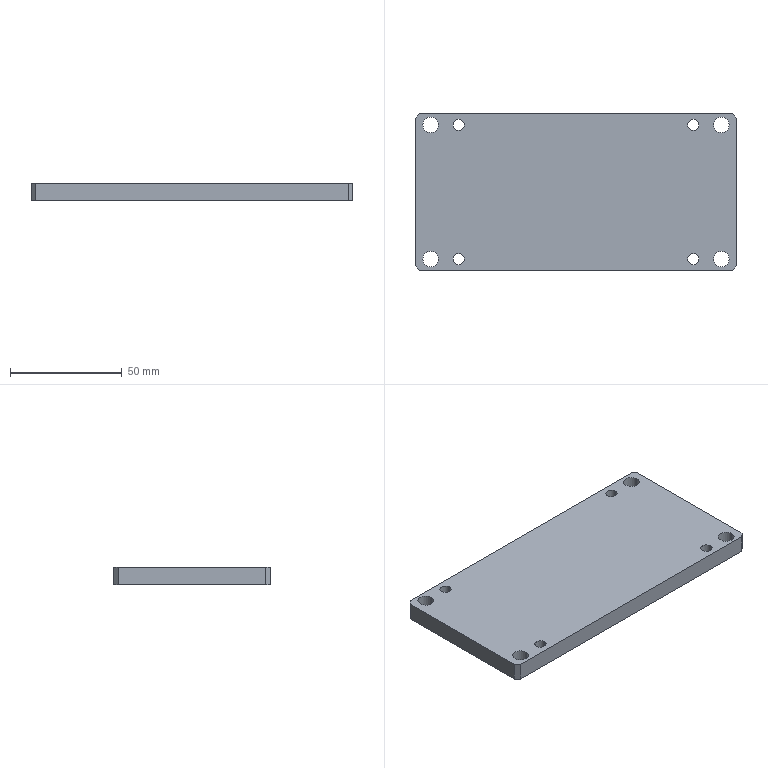Part | SolidWorks | features Chamfer 1, Extrusion 1, HoleWzd 1 | 1 solid | 26 faces | box 144 x 70 x 8 mm | volume 78716 mm3 | cylinder 16 | plane 10 | commonest cylinder face diameters 5 x8 7 x8
STEP:
#1=CARTESIAN_POINT('',(-55.,30.,0.));
#2=VERTEX_POINT('',#1);
#3=CARTESIAN_POINT('',(-50.,30.,0.));
#4=VERTEX_POINT('',#3);
#5=CARTESIAN_POINT('',(-52.5,30.,0.));
#6=DIRECTION('',(0.,0.,1.));
#7=DIRECTION('',(1.,0.,0.));
#8=AXIS2_PLACEMENT_3D('',#5,#6,#7);
#9=CIRCLE('',#8,2.5);
#10=EDGE_CURVE('',#2,#4,#9,.T.);
#11=ORIENTED_EDGE('',*,*,#10,.F.);
#12=CARTESIAN_POINT('',(-55.,30.,8.));
#13=VERTEX_POINT('',#12);
#14=CARTESIAN_POINT('',(-55.,30.,8.));
#15=DIRECTION('',(0.,0.,1.));
#16=VECTOR('',#15,1000.);
#17=LINE('',#14,#16);
#18=EDGE_CURVE('',#2,#13,#17,.T.);
#19=ORIENTED_EDGE('',*,*,#18,.T.);
#20=CARTESIAN_POINT('',(-50.,30.,8.));
#21=VERTEX_POINT('',#20);
#22=CARTESIAN_POINT('',(-52.5,30.,8.));
#23=DIRECTION('',(0.,0.,1.));
#24=DIRECTION('',(1.,0.,0.));
#25=AXIS2_PLACEMENT_3D('',#22,#23,#24);
#26=CIRCLE('',#25,2.5);
#27=EDGE_CURVE('',#13,#21,#26,.T.);
#28=ORIENTED_EDGE('',*,*,#27,.T.);
#29=CARTESIAN_POINT('',(-50.,30.,8.));
#30=DIRECTION('',(0.,0.,1.));
#31=VECTOR('',#30,1000.);
#32=LINE('',#29,#31);
#33=EDGE_CURVE('',#4,#21,#32,.T.);
#34=ORIENTED_EDGE('',*,*,#33,.F.);
#35=EDGE_LOOP('',(#11,#19,#28,#34));
#36=FACE_OUTER_BOUND('',#35,.T.);
#37=CARTESIAN_POINT('',(-52.5,30.,8.));
#38=DIRECTION('',(0.,0.,1.));
#39=DIRECTION('',(1.,0.,0.));
#40=AXIS2_PLACEMENT_3D('',#37,#38,#39);
#41=CYLINDRICAL_SURFACE('',#40,2.5);
#42=ADVANCED_FACE('',(#36),#41,.F.);
#43=CARTESIAN_POINT('',(-55.,-30.,0.));
#44=VERTEX_POINT('',#43);
#45=CARTESIAN_POINT('',(-50.,-30.,0.));
#46=VERTEX_POINT('',#45);
#47=CARTESIAN_POINT('',(-52.5,-30.,0.));
#48=DIRECTION('',(0.,0.,1.));
#49=DIRECTION('',(1.,0.,0.));
#50=AXIS2_PLACEMENT_3D('',#47,#48,#49);
#51=CIRCLE('',#50,2.5);
#52=EDGE_CURVE('',#44,#46,#51,.T.);
#53=ORIENTED_EDGE('',*,*,#52,.F.);
#54=CARTESIAN_POINT('',(-55.,-30.,8.));
#55=VERTEX_POINT('',#54);
#56=CARTESIAN_POINT('',(-55.,-30.,8.));
#57=DIRECTION('',(0.,0.,1.));
#58=VECTOR('',#57,1000.);
#59=LINE('',#56,#58);
#60=EDGE_CURVE('',#44,#55,#59,.T.);
#61=ORIENTED_EDGE('',*,*,#60,.T.);
#62=CARTESIAN_POINT('',(-50.,-30.,8.));
#63=VERTEX_POINT('',#62);
#64=CARTESIAN_POINT('',(-52.5,-30.,8.));
#65=DIRECTION('',(0.,0.,1.));
#66=DIRECTION('',(1.,0.,0.));
#67=AXIS2_PLACEMENT_3D('',#64,#65,#66);
#68=CIRCLE('',#67,2.5);
#69=EDGE_CURVE('',#55,#63,#68,.T.);
#70=ORIENTED_EDGE('',*,*,#69,.T.);
#71=CARTESIAN_POINT('',(-50.,-30.,8.));
#72=DIRECTION('',(0.,0.,1.));
#73=VECTOR('',#72,1000.);
#74=LINE('',#71,#73);
#75=EDGE_CURVE('',#46,#63,#74,.T.);
#76=ORIENTED_EDGE('',*,*,#75,.F.);
#77=EDGE_LOOP('',(#53,#61,#70,#76));
#78=FACE_OUTER_BOUND('',#77,.T.);
#79=CARTESIAN_POINT('',(-52.5,-30.,8.));
#80=DIRECTION('',(0.,0.,1.));
#81=DIRECTION('',(1.,0.,0.));
#82=AXIS2_PLACEMENT_3D('',#79,#80,#81);
#83=CYLINDRICAL_SURFACE('',#82,2.5);
#84=ADVANCED_FACE('',(#78),#83,.F.);
#85=CARTESIAN_POINT('',(50.,-30.,0.));
#86=VERTEX_POINT('',#85);
#87=CARTESIAN_POINT('',(55.,-30.,0.));
#88=VERTEX_POINT('',#87);
#89=CARTESIAN_POINT('',(52.5,-30.,0.));
#90=DIRECTION('',(0.,0.,1.));
#91=DIRECTION('',(1.,0.,0.));
#92=AXIS2_PLACEMENT_3D('',#89,#90,#91);
#93=CIRCLE('',#92,2.5);
#94=EDGE_CURVE('',#86,#88,#93,.T.);
#95=ORIENTED_EDGE('',*,*,#94,.F.);
#96=CARTESIAN_POINT('',(50.,-30.,8.));
#97=VERTEX_POINT('',#96);
#98=CARTESIAN_POINT('',(50.,-30.,8.));
#99=DIRECTION('',(0.,0.,1.));
#100=VECTOR('',#99,1000.);
#101=LINE('',#98,#100);
#102=EDGE_CURVE('',#86,#97,#101,.T.);
#103=ORIENTED_EDGE('',*,*,#102,.T.);
#104=CARTESIAN_POINT('',(55.,-30.,8.));
#105=VERTEX_POINT('',#104);
#106=CARTESIAN_POINT('',(52.5,-30.,8.));
#107=DIRECTION('',(0.,0.,1.));
#108=DIRECTION('',(1.,0.,0.));
#109=AXIS2_PLACEMENT_3D('',#106,#107,#108);
#110=CIRCLE('',#109,2.5);
#111=EDGE_CURVE('',#97,#105,#110,.T.);
#112=ORIENTED_EDGE('',*,*,#111,.T.);
#113=CARTESIAN_POINT('',(55.,-30.,8.));
#114=DIRECTION('',(0.,0.,1.));
#115=VECTOR('',#114,1000.);
#116=LINE('',#113,#115);
#117=EDGE_CURVE('',#88,#105,#116,.T.);
#118=ORIENTED_EDGE('',*,*,#117,.F.);
#119=EDGE_LOOP('',(#95,#103,#112,#118));
#120=FACE_OUTER_BOUND('',#119,.T.);
#121=CARTESIAN_POINT('',(52.5,-30.,8.));
#122=DIRECTION('',(0.,0.,1.));
#123=DIRECTION('',(1.,0.,0.));
#124=AXIS2_PLACEMENT_3D('',#121,#122,#123);
#125=CYLINDRICAL_SURFACE('',#124,2.5);
#126=ADVANCED_FACE('',(#120),#125,.F.);
#127=CARTESIAN_POINT('',(50.,30.,0.));
#128=VERTEX_POINT('',#127);
#129=CARTESIAN_POINT('',(55.,30.,0.));
#130=VERTEX_POINT('',#129);
#131=CARTESIAN_POINT('',(52.5,30.,0.));
#132=DIRECTION('',(0.,0.,1.));
#133=DIRECTION('',(1.,0.,0.));
#134=AXIS2_PLACEMENT_3D('',#131,#132,#133);
#135=CIRCLE('',#134,2.5);
#136=EDGE_CURVE('',#128,#130,#135,.T.);
#137=ORIENTED_EDGE('',*,*,#136,.F.);
#138=CARTESIAN_POINT('',(50.,30.,8.));
#139=VERTEX_POINT('',#138);
#140=CARTESIAN_POINT('',(50.,30.,8.));
#141=DIRECTION('',(0.,0.,1.));
#142=VECTOR('',#141,1000.);
#143=LINE('',#140,#142);
#144=EDGE_CURVE('',#128,#139,#143,.T.);
#145=ORIENTED_EDGE('',*,*,#144,.T.);
#146=CARTESIAN_POINT('',(55.,30.,8.));
#147=VERTEX_POINT('',#146);
#148=CARTESIAN_POINT('',(52.5,30.,8.));
#149=DIRECTION('',(0.,0.,1.));
#150=DIRECTION('',(1.,0.,0.));
#151=AXIS2_PLACEMENT_3D('',#148,#149,#150);
#152=CIRCLE('',#151,2.5);
#153=EDGE_CURVE('',#139,#147,#152,.T.);
#154=ORIENTED_EDGE('',*,*,#153,.T.);
#155=CARTESIAN_POINT('',(55.,30.,8.));
#156=DIRECTION('',(0.,0.,1.));
#157=VECTOR('',#156,1000.);
#158=LINE('',#155,#157);
#159=EDGE_CURVE('',#130,#147,#158,.T.);
#160=ORIENTED_EDGE('',*,*,#159,.F.);
#161=EDGE_LOOP('',(#137,#145,#154,#160));
#162=FACE_OUTER_BOUND('',#161,.T.);
#163=CARTESIAN_POINT('',(52.5,30.,8.));
#164=DIRECTION('',(0.,0.,1.));
#165=DIRECTION('',(1.,0.,0.));
#166=AXIS2_PLACEMENT_3D('',#163,#164,#165);
#167=CYLINDRICAL_SURFACE('',#166,2.5);
#168=ADVANCED_FACE('',(#162),#167,.F.);
#169=CARTESIAN_POINT('',(61.5,30.,8.));
#170=VERTEX_POINT('',#169);
#171=CARTESIAN_POINT('',(68.5,30.,8.));
#172=VERTEX_POINT('',#171);
#173=CARTESIAN_POINT('',(65.,30.,8.));
#174=DIRECTION('',(0.,0.,1.));
#175=DIRECTION('',(1.,0.,0.));
#176=AXIS2_PLACEMENT_3D('',#173,#174,#175);
#177=CIRCLE('',#176,3.5);
#178=EDGE_CURVE('',#170,#172,#177,.T.);
#179=ORIENTED_EDGE('',*,*,#178,.T.);
#180=CARTESIAN_POINT('',(68.5,30.,0.));
#181=VERTEX_POINT('',#180);
#182=CARTESIAN_POINT('',(68.5,30.,8.));
#183=DIRECTION('',(0.,0.,-1.));
#184=VECTOR('',#183,1000.);
#185=LINE('',#182,#184);
#186=EDGE_CURVE('',#172,#181,#185,.T.);
#187=ORIENTED_EDGE('',*,*,#186,.T.);
#188=CARTESIAN_POINT('',(61.5,30.,0.));
#189=VERTEX_POINT('',#188);
#190=CARTESIAN_POINT('',(65.,30.,0.));
#191=DIRECTION('',(0.,0.,1.));
#192=DIRECTION('',(1.,0.,0.));
#193=AXIS2_PLACEMENT_3D('',#190,#191,#192);
#194=CIRCLE('',#193,3.5);
#195=EDGE_CURVE('',#189,#181,#194,.T.);
#196=ORIENTED_EDGE('',*,*,#195,.F.);
#197=CARTESIAN_POINT('',(61.5,30.,8.));
#198=DIRECTION('',(0.,0.,-1.));
#199=VECTOR('',#198,1000.);
#200=LINE('',#197,#199);
#201=EDGE_CURVE('',#170,#189,#200,.T.);
#202=ORIENTED_EDGE('',*,*,#201,.F.);
#203=EDGE_LOOP('',(#179,#187,#196,#202));
#204=FACE_OUTER_BOUND('',#203,.T.);
#205=CARTESIAN_POINT('',(65.,30.,8.));
#206=DIRECTION('',(0.,0.,-1.));
#207=DIRECTION('',(-1.,0.,0.));
#208=AXIS2_PLACEMENT_3D('',#205,#206,#207);
#209=CYLINDRICAL_SURFACE('',#208,3.5);
#210=ADVANCED_FACE('',(#204),#209,.F.);
#211=CARTESIAN_POINT('',(61.5,-30.,8.));
#212=VERTEX_POINT('',#211);
#213=CARTESIAN_POINT('',(68.5,-30.,8.));
#214=VERTEX_POINT('',#213);
#215=CARTESIAN_POINT('',(65.,-30.,8.));
#216=DIRECTION('',(0.,0.,1.));
#217=DIRECTION('',(1.,0.,0.));
#218=AXIS2_PLACEMENT_3D('',#215,#216,#217);
#219=CIRCLE('',#218,3.5);
#220=EDGE_CURVE('',#212,#214,#219,.T.);
#221=ORIENTED_EDGE('',*,*,#220,.T.);
#222=CARTESIAN_POINT('',(68.5,-30.,0.));
#223=VERTEX_POINT('',#222);
#224=CARTESIAN_POINT('',(68.5,-30.,8.));
#225=DIRECTION('',(0.,0.,-1.));
#226=VECTOR('',#225,1000.);
#227=LINE('',#224,#226);
#228=EDGE_CURVE('',#214,#223,#227,.T.);
#229=ORIENTED_EDGE('',*,*,#228,.T.);
#230=CARTESIAN_POINT('',(61.5,-30.,0.));
#231=VERTEX_POINT('',#230);
#232=CARTESIAN_POINT('',(65.,-30.,0.));
#233=DIRECTION('',(0.,0.,1.));
#234=DIRECTION('',(1.,0.,0.));
#235=AXIS2_PLACEMENT_3D('',#232,#233,#234);
#236=CIRCLE('',#235,3.5);
#237=EDGE_CURVE('',#231,#223,#236,.T.);
#238=ORIENTED_EDGE('',*,*,#237,.F.);
#239=CARTESIAN_POINT('',(61.5,-30.,8.));
#240=DIRECTION('',(0.,0.,-1.));
#241=VECTOR('',#240,1000.);
#242=LINE('',#239,#241);
#243=EDGE_CURVE('',#212,#231,#242,.T.);
#244=ORIENTED_EDGE('',*,*,#243,.F.);
#245=EDGE_LOOP('',(#221,#229,#238,#244));
#246=FACE_OUTER_BOUND('',#245,.T.);
#247=CARTESIAN_POINT('',(65.,-30.,8.));
#248=DIRECTION('',(0.,0.,-1.));
#249=DIRECTION('',(-1.,0.,0.));
#250=AXIS2_PLACEMENT_3D('',#247,#248,#249);
#251=CYLINDRICAL_SURFACE('',#250,3.5);
#252=ADVANCED_FACE('',(#246),#251,.F.);
#253=CARTESIAN_POINT('',(-68.5,-30.,8.));
#254=VERTEX_POINT('',#253);
#255=CARTESIAN_POINT('',(-61.5,-30.,8.));
#256=VERTEX_POINT('',#255);
#257=CARTESIAN_POINT('',(-65.,-30.,8.));
#258=DIRECTION('',(0.,0.,1.));
#259=DIRECTION('',(1.,0.,0.));
#260=AXIS2_PLACEMENT_3D('',#257,#258,#259);
#261=CIRCLE('',#260,3.5);
#262=EDGE_CURVE('',#254,#256,#261,.T.);
#263=ORIENTED_EDGE('',*,*,#262,.T.);
#264=CARTESIAN_POINT('',(-61.5,-30.,0.));
#265=VERTEX_POINT('',#264);
#266=CARTESIAN_POINT('',(-61.5,-30.,8.));
#267=DIRECTION('',(0.,0.,-1.));
#268=VECTOR('',#267,1000.);
#269=LINE('',#266,#268);
#270=EDGE_CURVE('',#256,#265,#269,.T.);
#271=ORIENTED_EDGE('',*,*,#270,.T.);
#272=CARTESIAN_POINT('',(-68.5,-30.,0.));
#273=VERTEX_POINT('',#272);
#274=CARTESIAN_POINT('',(-65.,-30.,0.));
#275=DIRECTION('',(0.,0.,1.));
#276=DIRECTION('',(1.,0.,0.));
#277=AXIS2_PLACEMENT_3D('',#274,#275,#276);
#278=CIRCLE('',#277,3.5);
#279=EDGE_CURVE('',#273,#265,#278,.T.);
#280=ORIENTED_EDGE('',*,*,#279,.F.);
#281=CARTESIAN_POINT('',(-68.5,-30.,8.));
#282=DIRECTION('',(0.,0.,-1.));
#283=VECTOR('',#282,1000.);
#284=LINE('',#281,#283);
#285=EDGE_CURVE('',#254,#273,#284,.T.);
#286=ORIENTED_EDGE('',*,*,#285,.F.);
#287=EDGE_LOOP('',(#263,#271,#280,#286));
#288=FACE_OUTER_BOUND('',#287,.T.);
#289=CARTESIAN_POINT('',(-65.,-30.,8.));
#290=DIRECTION('',(0.,0.,-1.));
#291=DIRECTION('',(-1.,0.,0.));
#292=AXIS2_PLACEMENT_3D('',#289,#290,#291);
#293=CYLINDRICAL_SURFACE('',#292,3.5);
#294=ADVANCED_FACE('',(#288),#293,.F.);
#295=CARTESIAN_POINT('',(-68.5,30.,8.));
#296=VERTEX_POINT('',#295);
#297=CARTESIAN_POINT('',(-61.5,30.,8.));
#298=VERTEX_POINT('',#297);
#299=CARTESIAN_POINT('',(-65.,30.,8.));
#300=DIRECTION('',(0.,0.,1.));
#301=DIRECTION('',(1.,0.,0.));
#302=AXIS2_PLACEMENT_3D('',#299,#300,#301);
#303=CIRCLE('',#302,3.5);
#304=EDGE_CURVE('',#296,#298,#303,.T.);
#305=ORIENTED_EDGE('',*,*,#304,.T.);
#306=CARTESIAN_POINT('',(-61.5,30.,0.));
#307=VERTEX_POINT('',#306);
#308=CARTESIAN_POINT('',(-61.5,30.,8.));
#309=DIRECTION('',(0.,0.,-1.));
#310=VECTOR('',#309,1000.);
#311=LINE('',#308,#310);
#312=EDGE_CURVE('',#298,#307,#311,.T.);
#313=ORIENTED_EDGE('',*,*,#312,.T.);
#314=CARTESIAN_POINT('',(-68.5,30.,0.));
#315=VERTEX_POINT('',#314);
#316=CARTESIAN_POINT('',(-65.,30.,0.));
#317=DIRECTION('',(0.,0.,1.));
#318=DIRECTION('',(1.,0.,0.));
#319=AXIS2_PLACEMENT_3D('',#316,#317,#318);
#320=CIRCLE('',#319,3.5);
#321=EDGE_CURVE('',#315,#307,#320,.T.);
#322=ORIENTED_EDGE('',*,*,#321,.F.);
#323=CARTESIAN_POINT('',(-68.5,30.,8.));
#324=DIRECTION('',(0.,0.,-1.));
#325=VECTOR('',#324,1000.);
#326=LINE('',#323,#325);
#327=EDGE_CURVE('',#296,#315,#326,.T.);
#328=ORIENTED_EDGE('',*,*,#327,.F.);
#329=EDGE_LOOP('',(#305,#313,#322,#328));
#330=FACE_OUTER_BOUND('',#329,.T.);
#331=CARTESIAN_POINT('',(-65.,30.,8.));
#332=DIRECTION('',(0.,0.,-1.));
#333=DIRECTION('',(-1.,0.,0.));
#334=AXIS2_PLACEMENT_3D('',#331,#332,#333);
#335=CYLINDRICAL_SURFACE('',#334,3.5);
#336=ADVANCED_FACE('',(#330),#335,.F.);
#337=CARTESIAN_POINT('',(-70.,-35.,0.));
#338=VERTEX_POINT('',#337);
#339=CARTESIAN_POINT('',(70.,-35.,0.));
#340=VERTEX_POINT('',#339);
#341=CARTESIAN_POINT('',(0.,-35.,0.));
#342=DIRECTION('',(1.,0.,0.));
#343=VECTOR('',#342,1000.);
#344=LINE('',#341,#343);
#345=EDGE_CURVE('',#338,#340,#344,.T.);
#346=ORIENTED_EDGE('',*,*,#345,.T.);
#347=CARTESIAN_POINT('',(70.,-35.,8.));
#348=VERTEX_POINT('',#347);
#349=CARTESIAN_POINT('',(70.,-35.,8.));
#350=DIRECTION('',(0.,0.,1.));
#351=VECTOR('',#350,1000.);
#352=LINE('',#349,#351);
#353=EDGE_CURVE('',#340,#348,#352,.T.);
#354=ORIENTED_EDGE('',*,*,#353,.T.);
#355=CARTESIAN_POINT('',(-70.,-35.,8.));
#356=VERTEX_POINT('',#355);
#357=CARTESIAN_POINT('',(0.,-35.,8.));
#358=DIRECTION('',(1.,0.,0.));
#359=VECTOR('',#358,1000.);
#360=LINE('',#357,#359);
#361=EDGE_CURVE('',#356,#348,#360,.T.);
#362=ORIENTED_EDGE('',*,*,#361,.F.);
#363=CARTESIAN_POINT('',(-70.,-35.,0.));
#364=DIRECTION('',(0.,0.,-1.));
#365=VECTOR('',#364,1000.);
#366=LINE('',#363,#365);
#367=EDGE_CURVE('',#356,#338,#366,.T.);
#368=ORIENTED_EDGE('',*,*,#367,.T.);
#369=EDGE_LOOP('',(#346,#354,#362,#368));
#370=FACE_OUTER_BOUND('',#369,.T.);
#371=CARTESIAN_POINT('',(0.,-35.,8.));
#372=DIRECTION('',(0.,1.,0.));
#373=DIRECTION('',(0.,0.,1.));
#374=AXIS2_PLACEMENT_3D('',#371,#372,#373);
#375=PLANE('',#374);
#376=ADVANCED_FACE('',(#370),#375,.F.);
#377=CARTESIAN_POINT('',(72.,-33.,0.));
#378=VERTEX_POINT('',#377);
#379=CARTESIAN_POINT('',(72.,33.,0.));
#380=VERTEX_POINT('',#379);
#381=CARTESIAN_POINT('',(72.,0.,0.));
#382=DIRECTION('',(0.,1.,0.));
#383=VECTOR('',#382,1000.);
#384=LINE('',#381,#383);
#385=EDGE_CURVE('',#378,#380,#384,.T.);
#386=ORIENTED_EDGE('',*,*,#385,.T.);
#387=CARTESIAN_POINT('',(72.,33.,8.));
#388=VERTEX_POINT('',#387);
#389=CARTESIAN_POINT('',(72.,33.,8.));
#390=DIRECTION('',(0.,0.,1.));
#391=VECTOR('',#390,1000.);
#392=LINE('',#389,#391);
#393=EDGE_CURVE('',#380,#388,#392,.T.);
#394=ORIENTED_EDGE('',*,*,#393,.T.);
#395=CARTESIAN_POINT('',(72.,-33.,8.));
#396=VERTEX_POINT('',#395);
#397=CARTESIAN_POINT('',(72.,0.,8.));
#398=DIRECTION('',(0.,1.,0.));
#399=VECTOR('',#398,1000.);
#400=LINE('',#397,#399);
#401=EDGE_CURVE('',#396,#388,#400,.T.);
#402=ORIENTED_EDGE('',*,*,#401,.F.);
#403=CARTESIAN_POINT('',(72.,-33.,8.));
#404=DIRECTION('',(0.,0.,-1.));
#405=VECTOR('',#404,1000.);
#406=LINE('',#403,#405);
#407=EDGE_CURVE('',#396,#378,#406,.T.);
#408=ORIENTED_EDGE('',*,*,#407,.T.);
#409=EDGE_LOOP('',(#386,#394,#402,#408));
#410=FACE_OUTER_BOUND('',#409,.T.);
#411=CARTESIAN_POINT('',(72.,0.,8.));
#412=DIRECTION('',(-1.,0.,0.));
#413=DIRECTION('',(0.,0.,1.));
#414=AXIS2_PLACEMENT_3D('',#411,#412,#413);
#415=PLANE('',#414);
#416=ADVANCED_FACE('',(#410),#415,.F.);
#417=CARTESIAN_POINT('',(-70.,35.,8.));
#418=VERTEX_POINT('',#417);
#419=CARTESIAN_POINT('',(70.,35.,8.));
#420=VERTEX_POINT('',#419);
#421=CARTESIAN_POINT('',(0.,35.,8.));
#422=DIRECTION('',(1.,0.,0.));
#423=VECTOR('',#422,1000.);
#424=LINE('',#421,#423);
#425=EDGE_CURVE('',#418,#420,#424,.T.);
#426=ORIENTED_EDGE('',*,*,#425,.T.);
#427=CARTESIAN_POINT('',(70.,35.,0.));
#428=VERTEX_POINT('',#427);
#429=CARTESIAN_POINT('',(70.,35.,0.));
#430=DIRECTION('',(0.,0.,-1.));
#431=VECTOR('',#430,1000.);
#432=LINE('',#429,#431);
#433=EDGE_CURVE('',#420,#428,#432,.T.);
#434=ORIENTED_EDGE('',*,*,#433,.T.);
#435=CARTESIAN_POINT('',(-70.,35.,0.));
#436=VERTEX_POINT('',#435);
#437=CARTESIAN_POINT('',(0.,35.,0.));
#438=DIRECTION('',(1.,0.,0.));
#439=VECTOR('',#438,1000.);
#440=LINE('',#437,#439);
#441=EDGE_CURVE('',#436,#428,#440,.T.);
#442=ORIENTED_EDGE('',*,*,#441,.F.);
#443=CARTESIAN_POINT('',(-70.,35.,8.));
#444=DIRECTION('',(0.,0.,1.));
#445=VECTOR('',#444,1000.);
#446=LINE('',#443,#445);
#447=EDGE_CURVE('',#436,#418,#446,.T.);
#448=ORIENTED_EDGE('',*,*,#447,.T.);
#449=EDGE_LOOP('',(#426,#434,#442,#448));
#450=FACE_OUTER_BOUND('',#449,.T.);
#451=CARTESIAN_POINT('',(0.,35.,8.));
#452=DIRECTION('',(0.,1.,0.));
#453=DIRECTION('',(0.,0.,1.));
#454=AXIS2_PLACEMENT_3D('',#451,#452,#453);
#455=PLANE('',#454);
#456=ADVANCED_FACE('',(#450),#455,.T.);
#457=ORIENTED_EDGE('',*,*,#312,.F.);
#458=CARTESIAN_POINT('',(-65.,30.,8.));
#459=DIRECTION('',(0.,0.,1.));
#460=DIRECTION('',(1.,0.,0.));
#461=AXIS2_PLACEMENT_3D('',#458,#459,#460);
#462=CIRCLE('',#461,3.5);
#463=EDGE_CURVE('',#298,#296,#462,.T.);
#464=ORIENTED_EDGE('',*,*,#463,.T.);
#465=ORIENTED_EDGE('',*,*,#327,.T.);
#466=CARTESIAN_POINT('',(-65.,30.,0.));
#467=DIRECTION('',(0.,0.,1.));
#468=DIRECTION('',(1.,0.,0.));
#469=AXIS2_PLACEMENT_3D('',#466,#467,#468);
#470=CIRCLE('',#469,3.5);
#471=EDGE_CURVE('',#307,#315,#470,.T.);
#472=ORIENTED_EDGE('',*,*,#471,.F.);
#473=EDGE_LOOP('',(#457,#464,#465,#472));
#474=FACE_OUTER_BOUND('',#473,.T.);
#475=CARTESIAN_POINT('',(-65.,30.,8.));
#476=DIRECTION('',(0.,0.,-1.));
#477=DIRECTION('',(-1.,0.,0.));
#478=AXIS2_PLACEMENT_3D('',#475,#476,#477);
#479=CYLINDRICAL_SURFACE('',#478,3.5);
#480=ADVANCED_FACE('',(#474),#479,.F.);
#481=ORIENTED_EDGE('',*,*,#270,.F.);
#482=CARTESIAN_POINT('',(-65.,-30.,8.));
#483=DIRECTION('',(0.,0.,1.));
#484=DIRECTION('',(1.,0.,0.));
#485=AXIS2_PLACEMENT_3D('',#482,#483,#484);
#486=CIRCLE('',#485,3.5);
#487=EDGE_CURVE('',#256,#254,#486,.T.);
#488=ORIENTED_EDGE('',*,*,#487,.T.);
#489=ORIENTED_EDGE('',*,*,#285,.T.);
#490=CARTESIAN_POINT('',(-65.,-30.,0.));
#491=DIRECTION('',(0.,0.,1.));
#492=DIRECTION('',(1.,0.,0.));
#493=AXIS2_PLACEMENT_3D('',#490,#491,#492);
#494=CIRCLE('',#493,3.5);
#495=EDGE_CURVE('',#265,#273,#494,.T.);
#496=ORIENTED_EDGE('',*,*,#495,.F.);
#497=EDGE_LOOP('',(#481,#488,#489,#496));
#498=FACE_OUTER_BOUND('',#497,.T.);
#499=CARTESIAN_POINT('',(-65.,-30.,8.));
#500=DIRECTION('',(0.,0.,-1.));
#501=DIRECTION('',(-1.,0.,0.));
#502=AXIS2_PLACEMENT_3D('',#499,#500,#501);
#503=CYLINDRICAL_SURFACE('',#502,3.5);
#504=ADVANCED_FACE('',(#498),#503,.F.);
#505=ORIENTED_EDGE('',*,*,#228,.F.);
#506=CARTESIAN_POINT('',(65.,-30.,8.));
#507=DIRECTION('',(0.,0.,1.));
#508=DIRECTION('',(1.,0.,0.));
#509=AXIS2_PLACEMENT_3D('',#506,#507,#508);
#510=CIRCLE('',#509,3.5);
#511=EDGE_CURVE('',#214,#212,#510,.T.);
#512=ORIENTED_EDGE('',*,*,#511,.T.);
#513=ORIENTED_EDGE('',*,*,#243,.T.);
#514=CARTESIAN_POINT('',(65.,-30.,0.));
#515=DIRECTION('',(0.,0.,1.));
#516=DIRECTION('',(1.,0.,0.));
#517=AXIS2_PLACEMENT_3D('',#514,#515,#516);
#518=CIRCLE('',#517,3.5);
#519=EDGE_CURVE('',#223,#231,#518,.T.);
#520=ORIENTED_EDGE('',*,*,#519,.F.);
#521=EDGE_LOOP('',(#505,#512,#513,#520));
#522=FACE_OUTER_BOUND('',#521,.T.);
#523=CARTESIAN_POINT('',(65.,-30.,8.));
#524=DIRECTION('',(0.,0.,-1.));
#525=DIRECTION('',(-1.,0.,0.));
#526=AXIS2_PLACEMENT_3D('',#523,#524,#525);
#527=CYLINDRICAL_SURFACE('',#526,3.5);
#528=ADVANCED_FACE('',(#522),#527,.F.);
#529=ORIENTED_EDGE('',*,*,#186,.F.);
#530=CARTESIAN_POINT('',(65.,30.,8.));
#531=DIRECTION('',(0.,0.,1.));
#532=DIRECTION('',(1.,0.,0.));
#533=AXIS2_PLACEMENT_3D('',#530,#531,#532);
#534=CIRCLE('',#533,3.5);
#535=EDGE_CURVE('',#172,#170,#534,.T.);
#536=ORIENTED_EDGE('',*,*,#535,.T.);
#537=ORIENTED_EDGE('',*,*,#201,.T.);
#538=CARTESIAN_POINT('',(65.,30.,0.));
#539=DIRECTION('',(0.,0.,1.));
#540=DIRECTION('',(1.,0.,0.));
#541=AXIS2_PLACEMENT_3D('',#538,#539,#540);
#542=CIRCLE('',#541,3.5);
#543=EDGE_CURVE('',#181,#189,#542,.T.);
#544=ORIENTED_EDGE('',*,*,#543,.F.);
#545=EDGE_LOOP('',(#529,#536,#537,#544));
#546=FACE_OUTER_BOUND('',#545,.T.);
#547=CARTESIAN_POINT('',(65.,30.,8.));
#548=DIRECTION('',(0.,0.,-1.));
#549=DIRECTION('',(-1.,0.,0.));
#550=AXIS2_PLACEMENT_3D('',#547,#548,#549);
#551=CYLINDRICAL_SURFACE('',#550,3.5);
#552=ADVANCED_FACE('',(#546),#551,.F.);
#553=CARTESIAN_POINT('',(-72.,-33.,0.));
#554=VERTEX_POINT('',#553);
#555=CARTESIAN_POINT('',(-72.,33.,0.));
#556=VERTEX_POINT('',#555);
#557=CARTESIAN_POINT('',(-72.,0.,0.));
#558=DIRECTION('',(0.,1.,0.));
#559=VECTOR('',#558,1000.);
#560=LINE('',#557,#559);
#561=EDGE_CURVE('',#554,#556,#560,.T.);
#562=ORIENTED_EDGE('',*,*,#561,.F.);
#563=CARTESIAN_POINT('',(-72.,-33.,8.));
#564=VERTEX_POINT('',#563);
#565=CARTESIAN_POINT('',(-72.,-33.,8.));
#566=DIRECTION('',(0.,0.,1.));
#567=VECTOR('',#566,1000.);
#568=LINE('',#565,#567);
#569=EDGE_CURVE('',#554,#564,#568,.T.);
#570=ORIENTED_EDGE('',*,*,#569,.T.);
#571=CARTESIAN_POINT('',(-72.,33.,8.));
#572=VERTEX_POINT('',#571);
#573=CARTESIAN_POINT('',(-72.,0.,8.));
#574=DIRECTION('',(0.,1.,0.));
#575=VECTOR('',#574,1000.);
#576=LINE('',#573,#575);
#577=EDGE_CURVE('',#564,#572,#576,.T.);
#578=ORIENTED_EDGE('',*,*,#577,.T.);
#579=CARTESIAN_POINT('',(-72.,33.,8.));
#580=DIRECTION('',(0.,0.,-1.));
#581=VECTOR('',#580,1000.);
#582=LINE('',#579,#581);
#583=EDGE_CURVE('',#572,#556,#582,.T.);
#584=ORIENTED_EDGE('',*,*,#583,.T.);
#585=EDGE_LOOP('',(#562,#570,#578,#584));
#586=FACE_OUTER_BOUND('',#585,.T.);
#587=CARTESIAN_POINT('',(-72.,0.,8.));
#588=DIRECTION('',(-1.,0.,0.));
#589=DIRECTION('',(0.,0.,1.));
#590=AXIS2_PLACEMENT_3D('',#587,#588,#589);
#591=PLANE('',#590);
#592=ADVANCED_FACE('',(#586),#591,.T.);
#593=CARTESIAN_POINT('',(-52.5,30.,8.));
#594=DIRECTION('',(0.,0.,1.));
#595=DIRECTION('',(1.,0.,0.));
#596=AXIS2_PLACEMENT_3D('',#593,#594,#595);
#597=CIRCLE('',#596,2.5);
#598=EDGE_CURVE('',#21,#13,#597,.T.);
#599=ORIENTED_EDGE('',*,*,#598,.F.);
#600=ORIENTED_EDGE('',*,*,#27,.F.);
#601=EDGE_LOOP('',(#599,#600));
#602=FACE_BOUND('',#601,.T.);
#603=CARTESIAN_POINT('',(-52.5,-30.,8.));
#604=DIRECTION('',(0.,0.,1.));
#605=DIRECTION('',(1.,0.,0.));
#606=AXIS2_PLACEMENT_3D('',#603,#604,#605);
#607=CIRCLE('',#606,2.5);
#608=EDGE_CURVE('',#63,#55,#607,.T.);
#609=ORIENTED_EDGE('',*,*,#608,.F.);
#610=ORIENTED_EDGE('',*,*,#69,.F.);
#611=EDGE_LOOP('',(#609,#610));
#612=FACE_BOUND('',#611,.T.);
#613=CARTESIAN_POINT('',(52.5,-30.,8.));
#614=DIRECTION('',(0.,0.,1.));
#615=DIRECTION('',(1.,0.,0.));
#616=AXIS2_PLACEMENT_3D('',#613,#614,#615);
#617=CIRCLE('',#616,2.5);
#618=EDGE_CURVE('',#105,#97,#617,.T.);
#619=ORIENTED_EDGE('',*,*,#618,.F.);
#620=ORIENTED_EDGE('',*,*,#111,.F.);
#621=EDGE_LOOP('',(#619,#620));
#622=FACE_BOUND('',#621,.T.);
#623=CARTESIAN_POINT('',(52.5,30.,8.));
#624=DIRECTION('',(0.,0.,1.));
#625=DIRECTION('',(1.,0.,0.));
#626=AXIS2_PLACEMENT_3D('',#623,#624,#625);
#627=CIRCLE('',#626,2.5);
#628=EDGE_CURVE('',#147,#139,#627,.T.);
#629=ORIENTED_EDGE('',*,*,#628,.F.);
#630=ORIENTED_EDGE('',*,*,#153,.F.);
#631=EDGE_LOOP('',(#629,#630));
#632=FACE_BOUND('',#631,.T.);
#633=ORIENTED_EDGE('',*,*,#178,.F.);
#634=ORIENTED_EDGE('',*,*,#535,.F.);
#635=EDGE_LOOP('',(#633,#634));
#636=FACE_BOUND('',#635,.T.);
#637=ORIENTED_EDGE('',*,*,#220,.F.);
#638=ORIENTED_EDGE('',*,*,#511,.F.);
#639=EDGE_LOOP('',(#637,#638));
#640=FACE_BOUND('',#639,.T.);
#641=ORIENTED_EDGE('',*,*,#262,.F.);
#642=ORIENTED_EDGE('',*,*,#487,.F.);
#643=EDGE_LOOP('',(#641,#642));
#644=FACE_BOUND('',#643,.T.);
#645=ORIENTED_EDGE('',*,*,#304,.F.);
#646=ORIENTED_EDGE('',*,*,#463,.F.);
#647=EDGE_LOOP('',(#645,#646));
#648=FACE_BOUND('',#647,.T.);
#649=ORIENTED_EDGE('',*,*,#401,.T.);
#650=CARTESIAN_POINT('',(52.5,52.5,8.));
#651=DIRECTION('',(-0.7071,0.7071,0.));
#652=VECTOR('',#651,1000.);
#653=LINE('',#650,#652);
#654=EDGE_CURVE('',#388,#420,#653,.T.);
#655=ORIENTED_EDGE('',*,*,#654,.T.);
#656=ORIENTED_EDGE('',*,*,#425,.F.);
#657=CARTESIAN_POINT('',(-52.5,52.5,8.));
#658=DIRECTION('',(-0.7071,-0.7071,0.));
#659=VECTOR('',#658,1000.);
#660=LINE('',#657,#659);
#661=EDGE_CURVE('',#418,#572,#660,.T.);
#662=ORIENTED_EDGE('',*,*,#661,.T.);
#663=ORIENTED_EDGE('',*,*,#577,.F.);
#664=CARTESIAN_POINT('',(-52.5,-52.5,8.));
#665=DIRECTION('',(0.7071,-0.7071,0.));
#666=VECTOR('',#665,1000.);
#667=LINE('',#664,#666);
#668=EDGE_CURVE('',#564,#356,#667,.T.);
#669=ORIENTED_EDGE('',*,*,#668,.T.);
#670=ORIENTED_EDGE('',*,*,#361,.T.);
#671=CARTESIAN_POINT('',(52.5,-52.5,8.));
#672=DIRECTION('',(0.7071,0.7071,0.));
#673=VECTOR('',#672,1000.);
#674=LINE('',#671,#673);
#675=EDGE_CURVE('',#348,#396,#674,.T.);
#676=ORIENTED_EDGE('',*,*,#675,.T.);
#677=EDGE_LOOP('',(#649,#655,#656,#662,#663,#669,#670,#676));
#678=FACE_OUTER_BOUND('',#677,.T.);
#679=CARTESIAN_POINT('',(0.,0.,8.));
#680=DIRECTION('',(0.,0.,1.));
#681=DIRECTION('',(1.,0.,0.));
#682=AXIS2_PLACEMENT_3D('',#679,#680,#681);
#683=PLANE('',#682);
#684=ADVANCED_FACE('',(#602,#612,#622,#632,#636,#640,#644,#648,#678),#683,.T.);
#685=CARTESIAN_POINT('',(-52.5,30.,0.));
#686=DIRECTION('',(0.,0.,1.));
#687=DIRECTION('',(1.,0.,0.));
#688=AXIS2_PLACEMENT_3D('',#685,#686,#687);
#689=CIRCLE('',#688,2.5);
#690=EDGE_CURVE('',#4,#2,#689,.T.);
#691=ORIENTED_EDGE('',*,*,#690,.T.);
#692=ORIENTED_EDGE('',*,*,#10,.T.);
#693=EDGE_LOOP('',(#691,#692));
#694=FACE_BOUND('',#693,.T.);
#695=CARTESIAN_POINT('',(-52.5,-30.,0.));
#696=DIRECTION('',(0.,0.,1.));
#697=DIRECTION('',(1.,0.,0.));
#698=AXIS2_PLACEMENT_3D('',#695,#696,#697);
#699=CIRCLE('',#698,2.5);
#700=EDGE_CURVE('',#46,#44,#699,.T.);
#701=ORIENTED_EDGE('',*,*,#700,.T.);
#702=ORIENTED_EDGE('',*,*,#52,.T.);
#703=EDGE_LOOP('',(#701,#702));
#704=FACE_BOUND('',#703,.T.);
#705=CARTESIAN_POINT('',(52.5,-30.,0.));
#706=DIRECTION('',(0.,0.,1.));
#707=DIRECTION('',(1.,0.,0.));
#708=AXIS2_PLACEMENT_3D('',#705,#706,#707);
#709=CIRCLE('',#708,2.5);
#710=EDGE_CURVE('',#88,#86,#709,.T.);
#711=ORIENTED_EDGE('',*,*,#710,.T.);
#712=ORIENTED_EDGE('',*,*,#94,.T.);
#713=EDGE_LOOP('',(#711,#712));
#714=FACE_BOUND('',#713,.T.);
#715=CARTESIAN_POINT('',(52.5,30.,0.));
#716=DIRECTION('',(0.,0.,1.));
#717=DIRECTION('',(1.,0.,0.));
#718=AXIS2_PLACEMENT_3D('',#715,#716,#717);
#719=CIRCLE('',#718,2.5);
#720=EDGE_CURVE('',#130,#128,#719,.T.);
#721=ORIENTED_EDGE('',*,*,#720,.T.);
#722=ORIENTED_EDGE('',*,*,#136,.T.);
#723=EDGE_LOOP('',(#721,#722));
#724=FACE_BOUND('',#723,.T.);
#725=ORIENTED_EDGE('',*,*,#195,.T.);
#726=ORIENTED_EDGE('',*,*,#543,.T.);
#727=EDGE_LOOP('',(#725,#726));
#728=FACE_BOUND('',#727,.T.);
#729=ORIENTED_EDGE('',*,*,#237,.T.);
#730=ORIENTED_EDGE('',*,*,#519,.T.);
#731=EDGE_LOOP('',(#729,#730));
#732=FACE_BOUND('',#731,.T.);
#733=ORIENTED_EDGE('',*,*,#279,.T.);
#734=ORIENTED_EDGE('',*,*,#495,.T.);
#735=EDGE_LOOP('',(#733,#734));
#736=FACE_BOUND('',#735,.T.);
#737=ORIENTED_EDGE('',*,*,#321,.T.);
#738=ORIENTED_EDGE('',*,*,#471,.T.);
#739=EDGE_LOOP('',(#737,#738));
#740=FACE_BOUND('',#739,.T.);
#741=ORIENTED_EDGE('',*,*,#441,.T.);
#742=CARTESIAN_POINT('',(70.,35.,0.));
#743=DIRECTION('',(0.7071,-0.7071,0.));
#744=VECTOR('',#743,1000.);
#745=LINE('',#742,#744);
#746=EDGE_CURVE('',#428,#380,#745,.T.);
#747=ORIENTED_EDGE('',*,*,#746,.T.);
#748=ORIENTED_EDGE('',*,*,#385,.F.);
#749=CARTESIAN_POINT('',(72.,-33.,0.));
#750=DIRECTION('',(-0.7071,-0.7071,0.));
#751=VECTOR('',#750,1000.);
#752=LINE('',#749,#751);
#753=EDGE_CURVE('',#378,#340,#752,.T.);
#754=ORIENTED_EDGE('',*,*,#753,.T.);
#755=ORIENTED_EDGE('',*,*,#345,.F.);
#756=CARTESIAN_POINT('',(-70.,-35.,0.));
#757=DIRECTION('',(-0.7071,0.7071,0.));
#758=VECTOR('',#757,1000.);
#759=LINE('',#756,#758);
#760=EDGE_CURVE('',#338,#554,#759,.T.);
#761=ORIENTED_EDGE('',*,*,#760,.T.);
#762=ORIENTED_EDGE('',*,*,#561,.T.);
#763=CARTESIAN_POINT('',(-72.,33.,0.));
#764=DIRECTION('',(0.7071,0.7071,0.));
#765=VECTOR('',#764,1000.);
#766=LINE('',#763,#765);
#767=EDGE_CURVE('',#556,#436,#766,.T.);
#768=ORIENTED_EDGE('',*,*,#767,.T.);
#769=EDGE_LOOP('',(#741,#747,#748,#754,#755,#761,#762,#768));
#770=FACE_OUTER_BOUND('',#769,.T.);
#771=CARTESIAN_POINT('',(0.,0.,0.));
#772=DIRECTION('',(0.,0.,1.));
#773=DIRECTION('',(1.,0.,0.));
#774=AXIS2_PLACEMENT_3D('',#771,#772,#773);
#775=PLANE('',#774);
#776=ADVANCED_FACE('',(#694,#704,#714,#724,#728,#732,#736,#740,#770),#775,.F.);
#777=ORIENTED_EDGE('',*,*,#654,.F.);
#778=ORIENTED_EDGE('',*,*,#393,.F.);
#779=ORIENTED_EDGE('',*,*,#746,.F.);
#780=ORIENTED_EDGE('',*,*,#433,.F.);
#781=EDGE_LOOP('',(#777,#778,#779,#780));
#782=FACE_OUTER_BOUND('',#781,.T.);
#783=CARTESIAN_POINT('',(70.,35.,8.));
#784=DIRECTION('',(0.7071,0.7071,0.));
#785=DIRECTION('',(0.,0.,1.));
#786=AXIS2_PLACEMENT_3D('',#783,#784,#785);
#787=PLANE('',#786);
#788=ADVANCED_FACE('',(#782),#787,.T.);
#789=ORIENTED_EDGE('',*,*,#675,.F.);
#790=ORIENTED_EDGE('',*,*,#353,.F.);
#791=ORIENTED_EDGE('',*,*,#753,.F.);
#792=ORIENTED_EDGE('',*,*,#407,.F.);
#793=EDGE_LOOP('',(#789,#790,#791,#792));
#794=FACE_OUTER_BOUND('',#793,.T.);
#795=CARTESIAN_POINT('',(72.,-33.,8.));
#796=DIRECTION('',(-0.7071,0.7071,0.));
#797=DIRECTION('',(0.,0.,-1.));
#798=AXIS2_PLACEMENT_3D('',#795,#796,#797);
#799=PLANE('',#798);
#800=ADVANCED_FACE('',(#794),#799,.F.);
#801=ORIENTED_EDGE('',*,*,#668,.F.);
#802=ORIENTED_EDGE('',*,*,#569,.F.);
#803=ORIENTED_EDGE('',*,*,#760,.F.);
#804=ORIENTED_EDGE('',*,*,#367,.F.);
#805=EDGE_LOOP('',(#801,#802,#803,#804));
#806=FACE_OUTER_BOUND('',#805,.T.);
#807=CARTESIAN_POINT('',(-70.,-35.,8.));
#808=DIRECTION('',(-0.7071,-0.7071,0.));
#809=DIRECTION('',(0.,0.,1.));
#810=AXIS2_PLACEMENT_3D('',#807,#808,#809);
#811=PLANE('',#810);
#812=ADVANCED_FACE('',(#806),#811,.T.);
#813=ORIENTED_EDGE('',*,*,#661,.F.);
#814=ORIENTED_EDGE('',*,*,#447,.F.);
#815=ORIENTED_EDGE('',*,*,#767,.F.);
#816=ORIENTED_EDGE('',*,*,#583,.F.);
#817=EDGE_LOOP('',(#813,#814,#815,#816));
#818=FACE_OUTER_BOUND('',#817,.T.);
#819=CARTESIAN_POINT('',(-72.,33.,8.));
#820=DIRECTION('',(0.7071,-0.7071,0.));
#821=DIRECTION('',(0.,0.,-1.));
#822=AXIS2_PLACEMENT_3D('',#819,#820,#821);
#823=PLANE('',#822);
#824=ADVANCED_FACE('',(#818),#823,.F.);
#825=ORIENTED_EDGE('',*,*,#144,.F.);
#826=ORIENTED_EDGE('',*,*,#720,.F.);
#827=ORIENTED_EDGE('',*,*,#159,.T.);
#828=ORIENTED_EDGE('',*,*,#628,.T.);
#829=EDGE_LOOP('',(#825,#826,#827,#828));
#830=FACE_OUTER_BOUND('',#829,.T.);
#831=CARTESIAN_POINT('',(52.5,30.,8.));
#832=DIRECTION('',(0.,0.,1.));
#833=DIRECTION('',(1.,0.,0.));
#834=AXIS2_PLACEMENT_3D('',#831,#832,#833);
#835=CYLINDRICAL_SURFACE('',#834,2.5);
#836=ADVANCED_FACE('',(#830),#835,.F.);
#837=ORIENTED_EDGE('',*,*,#102,.F.);
#838=ORIENTED_EDGE('',*,*,#710,.F.);
#839=ORIENTED_EDGE('',*,*,#117,.T.);
#840=ORIENTED_EDGE('',*,*,#618,.T.);
#841=EDGE_LOOP('',(#837,#838,#839,#840));
#842=FACE_OUTER_BOUND('',#841,.T.);
#843=CARTESIAN_POINT('',(52.5,-30.,8.));
#844=DIRECTION('',(0.,0.,1.));
#845=DIRECTION('',(1.,0.,0.));
#846=AXIS2_PLACEMENT_3D('',#843,#844,#845);
#847=CYLINDRICAL_SURFACE('',#846,2.5);
#848=ADVANCED_FACE('',(#842),#847,.F.);
#849=ORIENTED_EDGE('',*,*,#60,.F.);
#850=ORIENTED_EDGE('',*,*,#700,.F.);
#851=ORIENTED_EDGE('',*,*,#75,.T.);
#852=ORIENTED_EDGE('',*,*,#608,.T.);
#853=EDGE_LOOP('',(#849,#850,#851,#852));
#854=FACE_OUTER_BOUND('',#853,.T.);
#855=CARTESIAN_POINT('',(-52.5,-30.,8.));
#856=DIRECTION('',(0.,0.,1.));
#857=DIRECTION('',(1.,0.,0.));
#858=AXIS2_PLACEMENT_3D('',#855,#856,#857);
#859=CYLINDRICAL_SURFACE('',#858,2.5);
#860=ADVANCED_FACE('',(#854),#859,.F.);
#861=ORIENTED_EDGE('',*,*,#18,.F.);
#862=ORIENTED_EDGE('',*,*,#690,.F.);
#863=ORIENTED_EDGE('',*,*,#33,.T.);
#864=ORIENTED_EDGE('',*,*,#598,.T.);
#865=EDGE_LOOP('',(#861,#862,#863,#864));
#866=FACE_OUTER_BOUND('',#865,.T.);
#867=CARTESIAN_POINT('',(-52.5,30.,8.));
#868=DIRECTION('',(0.,0.,1.));
#869=DIRECTION('',(1.,0.,0.));
#870=AXIS2_PLACEMENT_3D('',#867,#868,#869);
#871=CYLINDRICAL_SURFACE('',#870,2.5);
#872=ADVANCED_FACE('',(#866),#871,.F.);
#873=CLOSED_SHELL('',(#42,#84,#126,#168,#210,#252,#294,#336,#376,#416,#456,#480,#504,#528,#552,#592,#684,#776,#788,#800,#812,#824,#836,#848,#860,#872));
#874=MANIFOLD_SOLID_BREP('',#873);
#875=CARTESIAN_POINT('',(0.,0.,0.));
#876=DIRECTION('',(0.,0.,1.));
#877=DIRECTION('',(1.,0.,0.));
#878=AXIS2_PLACEMENT_3D('',#875,#876,#877);
#879=(LENGTH_UNIT()NAMED_UNIT(*)SI_UNIT(.MILLI.,.METRE.));
#880=UNCERTAINTY_MEASURE_WITH_UNIT(LENGTH_MEASURE(0.00001),#879,'','');
#881=(NAMED_UNIT(*)PLANE_ANGLE_UNIT()SI_UNIT($,.RADIAN.));
#882=(NAMED_UNIT(*)SI_UNIT($,.STERADIAN.)SOLID_ANGLE_UNIT());
#883=(GEOMETRIC_REPRESENTATION_CONTEXT(3)GLOBAL_UNCERTAINTY_ASSIGNED_CONTEXT((#880))GLOBAL_UNIT_ASSIGNED_CONTEXT((#879,#881,#882))REPRESENTATION_CONTEXT('',''));
#884=ADVANCED_BREP_SHAPE_REPRESENTATION('',(#874,#878),#883);